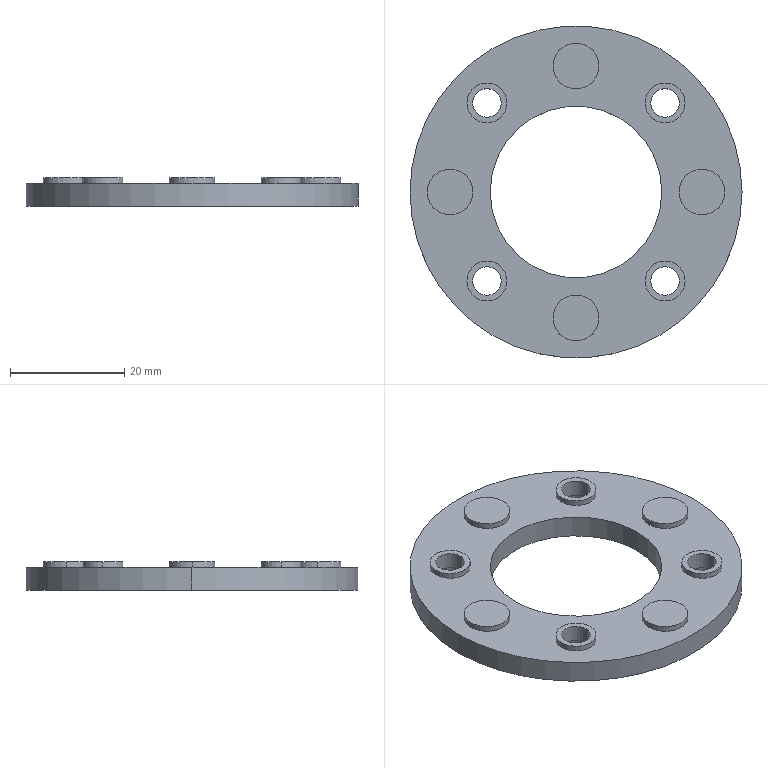Part | SolidWorks | features ICE 6, CirPattern 2, Extrusion 1 | 1 solid | 62 faces | box 58 x 58 x 5 mm | volume 7199 mm3 | cylinder 44 | plane 18 | commonest cylinder face diameters 5 x16 7 x16 8 x8 30 x2 58 x2